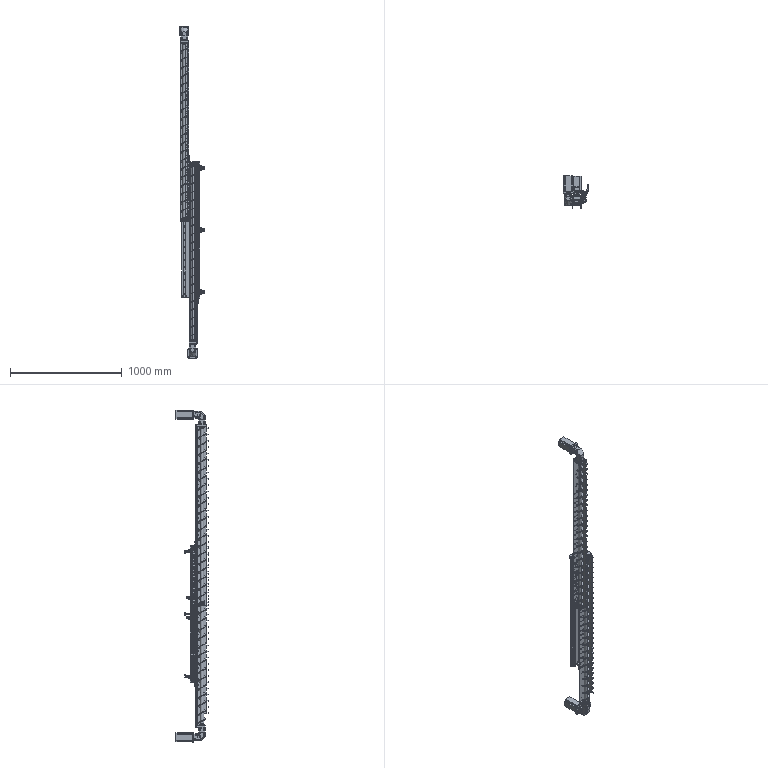Part | SolidWorks | features InContextFeatHolder 20 | 163 solids | 12191 faces | volume 13765877 mm3 | plane 6579 | cylinder 4440 | cone 756 | torus 184 | spline 166 | sphere 66 | commonest cylinder face diameters 1 x704 0.2 x340 6.8 x288 2 x284 4.2 x216 6 x214